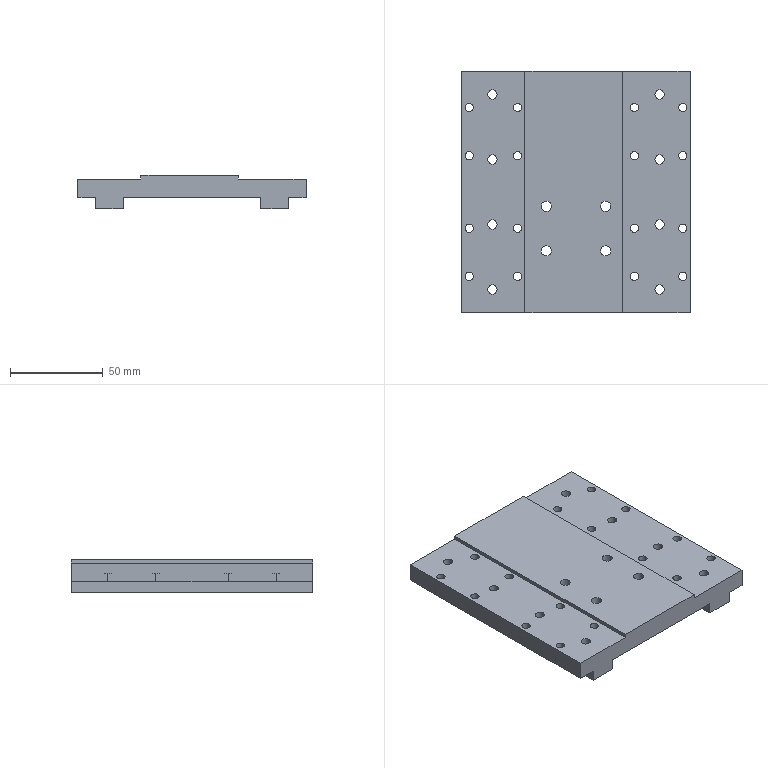NC program | NX | posted with a generic post | part box 123 x 130 x 18 mm
Lines 1 to 1849 of 2087, first 1534 of 1829 lines:
N10 G17 G21 G94 G90
(DRILLING , TOOL : D6A45)
N12 T01 M6
N14 G54
N16 G17 G0 G90 X-30.25 Y45.5 S5000 M3
N18 G43 Z30. H1
N20 G94 G81 G98 Z-1. F350. R3.
N22 X-43.75 Y52.5
N24 X-56.25 Y45.5
N26 Y19.5
N28 X-43.75 Y17.5
N30 X-30.25 Y19.5
N32 X-14.75 Y-7.7
N34 X-30.25 Y-19.5
N36 X-43.75 Y-17.5
N38 X-56.25 Y-19.5
N40 Y-45.5
N42 X-43.75 Y-52.5
N44 X-30.25 Y-45.5
N46 X-14.75 Y-31.7
N48 X17.25
N50 X32.75 Y-45.5
N52 X46.25 Y-52.5
N54 X58.75 Y-45.5
N56 Y-19.5
N58 X46.25 Y-17.5
N60 X32.75 Y-19.5
N62 X17.25 Y-7.7
N64 X32.75 Y19.5
N66 X46.25 Y17.5
N68 X58.75 Y19.5
N70 Y45.5
N72 X46.25 Y52.5
N74 X32.75 Y45.5
N76 G80
N78 G0 X32.75 Y45.5 Z30.
N80 M5
(DRILLING_COPY_COPY , TOOL : 5.5ZT)
N82 T09 M6
N84 G54
N86 G17 G0 G90 X-14.75 Y-7.7 S2000 M3
N88 G43 Z30. H9
N90 G94 G83 G98 Z-9.652 F300. Q2. R3.
N92 Y-31.7
N94 X17.25
N96 Y-7.7
N98 G80
N100 G0 X17.25 Y-7.7 Z30.
N102 M5
(DRILLING_COPY_COPY_COPY , TOOL : 5.0ZT)
N104 T16 M6
N106 G54
N108 G17 G0 G90 X46.25 Y-52.5 S2000 M3
N110 G43 Z30. H16
N112 G94 G83 G98 Z-21.002 F300. Q2. R3.
N114 Y-17.5
N116 Y17.5
N118 Y52.5
N120 X-43.75
N122 Y17.5
N124 Y-17.5
N126 Y-52.5
N128 G80
N130 G0 X-43.75 Y-52.5 Z30.
N132 M5
(DRILLING_COPY_COPY_COPY_COPY , TOOL : 4.5ZT)
N134 T08 M6
N136 G54
N138 G17 G0 G90 X32.75 Y-19.5 S2000 M3
N140 G43 Z30. H8
N142 G94 G83 G98 Z-10.352 F300. Q2. R3.
N144 Y-45.5
N146 X58.75
N148 Y-19.5
N150 Y19.5
N152 Y45.5
N154 X32.75
N156 Y19.5
N158 X-30.25
N160 Y45.5
N162 X-56.25
N164 Y19.5
N166 Y-19.5
N168 X-30.25
N170 Y-45.5
N172 X-56.25
N174 G80
N176 G0 X-56.25 Y-45.5 Z30.
N178 M5
(ZLEVEL_PROFILE , TOOL : D10)
N180 T15 M6
N182 G54
N184 G17 G0 G90 X-65.35 Y-47.067 S9500 M3
N186 G43 Z30. H15
N188 Z1.5
N190 G94 G1 Y0. Z-0.967 F1000.
N192 Y65. F3000.
N194 G2 X-60.25 Y70.1 R5.1
N196 G1 X62.75
N198 G2 X67.85 Y65. R5.1
N200 G1 Y-65.
N202 G2 X62.75 Y-70.1 R5.1
N204 G1 X-60.25
N206 G2 X-65.35 Y-65. R5.1
N208 G1 Y0.
N210 Y65. Z-1.083
N212 X-65.325 Y65.5 Z-1.084
N214 X-65.252 Y65.995 Z-1.085
N216 X-65.13 Y66.48 Z-1.086
N218 X-64.962 Y66.952 Z-1.087
N220 X-64.748 Y67.404 Z-1.088
N222 X-64.49 Y67.833 Z-1.089
N224 X-64.192 Y68.235 Z-1.09
N226 X-63.856 Y68.606 Z-1.091
N228 X-63.485 Y68.942 Z-1.092
N230 X-63.083 Y69.24
N232 X-62.654 Y69.498 Z-1.093
N234 X-62.202 Y69.712 Z-1.094
N236 X-61.73 Y69.88 Z-1.095
N238 X-61.245 Y70.002 Z-1.096
N240 X-60.75 Y70.075 Z-1.097
N242 X-60.25 Y70.1 Z-1.098
N244 X62.75 Z-1.319
N246 X63.25 Y70.075 Z-1.32
N248 X63.745 Y70.002 Z-1.321
N250 X64.23 Y69.88 Z-1.322
N252 X64.702 Y69.712
N254 X65.154 Y69.498 Z-1.323
N256 X65.583 Y69.24 Z-1.324
N258 X65.985 Y68.942 Z-1.325
N260 X66.356 Y68.606 Z-1.326
N262 X66.692 Y68.235 Z-1.327
N264 X66.99 Y67.833 Z-1.328
N266 X67.248 Y67.404 Z-1.329
N268 X67.462 Y66.952 Z-1.33
N270 X67.63 Y66.48 Z-1.331
N272 X67.752 Y65.995
N274 X67.825 Y65.5 Z-1.332
N276 X67.85 Y65. Z-1.333
N278 Y-65. Z-1.567
N280 X67.825 Y-65.5 Z-1.568
N282 X67.752 Y-65.995 Z-1.569
N284 X67.63 Y-66.48
N286 X67.462 Y-66.952 Z-1.57
N288 X67.248 Y-67.404 Z-1.571
N290 X66.99 Y-67.833 Z-1.572
N292 X66.692 Y-68.235 Z-1.573
N294 X66.356 Y-68.606 Z-1.574
N296 X65.985 Y-68.942 Z-1.575
N298 X65.583 Y-69.24 Z-1.576
N300 X65.154 Y-69.498 Z-1.577
N302 X64.702 Y-69.712 Z-1.578
N304 X64.23 Y-69.88
N306 X63.745 Y-70.002 Z-1.579
N308 X63.25 Y-70.075 Z-1.58
N310 X62.75 Y-70.1 Z-1.581
N312 X-60.25 Z-1.802
N314 X-60.75 Y-70.075 Z-1.803
N316 X-61.245 Y-70.002 Z-1.804
N318 X-61.73 Y-69.88 Z-1.805
N320 X-62.202 Y-69.712 Z-1.806
N322 X-62.654 Y-69.498 Z-1.807
N324 X-63.083 Y-69.24 Z-1.808
N326 X-63.485 Y-68.942
N328 X-63.856 Y-68.606 Z-1.809
N330 X-64.192 Y-68.235 Z-1.81
N332 X-64.49 Y-67.833 Z-1.811
N334 X-64.748 Y-67.404 Z-1.812
N336 X-64.962 Y-66.952 Z-1.813
N338 X-65.13 Y-66.48 Z-1.814
N340 X-65.252 Y-65.995 Z-1.815
N342 X-65.325 Y-65.5 Z-1.816
N344 X-65.35 Y-65. Z-1.817
N346 Y0. Z-1.933
N348 Y65. Z-2.05
N350 X-65.325 Y65.5 Z-2.051
N352 X-65.252 Y65.995 Z-2.052
N354 X-65.13 Y66.48 Z-2.053
N356 X-64.962 Y66.952 Z-2.054
N358 X-64.748 Y67.404 Z-2.055
N360 X-64.49 Y67.833 Z-2.056
N362 X-64.192 Y68.235
N364 X-63.856 Y68.606 Z-2.057
N366 X-63.485 Y68.942 Z-2.058
N368 X-63.083 Y69.24 Z-2.059
N370 X-62.654 Y69.498 Z-2.06
N372 X-62.202 Y69.712 Z-2.061
N374 X-61.73 Y69.88 Z-2.062
N376 X-61.245 Y70.002 Z-2.063
N378 X-60.75 Y70.075 Z-2.064
N380 X-60.25 Y70.1
N382 X62.75 Z-2.286
N384 X63.25 Y70.075
N386 X63.745 Y70.002 Z-2.287
N388 X64.23 Y69.88 Z-2.288
N390 X64.702 Y69.712 Z-2.289
N392 X65.154 Y69.498 Z-2.29
N394 X65.583 Y69.24 Z-2.291
N396 X65.985 Y68.942 Z-2.292
N398 X66.356 Y68.606 Z-2.293
N400 X66.692 Y68.235 Z-2.294
N402 X66.99 Y67.833
N404 X67.248 Y67.404 Z-2.295
N406 X67.462 Y66.952 Z-2.296
N408 X67.63 Y66.48 Z-2.297
N410 X67.752 Y65.995 Z-2.298
N412 X67.825 Y65.5 Z-2.299
N414 X67.85 Y65. Z-2.3
N416 Y-65. Z-2.533
N418 X67.825 Y-65.5 Z-2.534
N420 X67.752 Y-65.995 Z-2.535
N422 X67.63 Y-66.48 Z-2.536
N424 X67.462 Y-66.952 Z-2.537
N426 X67.248 Y-67.404 Z-2.538
N428 X66.99 Y-67.833 Z-2.539
N430 X66.692 Y-68.235 Z-2.54
N432 X66.356 Y-68.606 Z-2.541
N434 X65.985 Y-68.942 Z-2.542
N436 X65.583 Y-69.24
N438 X65.154 Y-69.498 Z-2.543
N440 X64.702 Y-69.712 Z-2.544
N442 X64.23 Y-69.88 Z-2.545
N444 X63.745 Y-70.002 Z-2.546
N446 X63.25 Y-70.075 Z-2.547
N448 X62.75 Y-70.1 Z-2.548
N450 X-60.25 Z-2.769
N452 X-60.75 Y-70.075 Z-2.77
N454 X-61.245 Y-70.002 Z-2.771
N456 X-61.73 Y-69.88 Z-2.772
N458 X-62.202 Y-69.712
N460 X-62.654 Y-69.498 Z-2.773
N462 X-63.083 Y-69.24 Z-2.774
N464 X-63.485 Y-68.942 Z-2.775
N466 X-63.856 Y-68.606 Z-2.776
N468 X-64.192 Y-68.235 Z-2.777
N470 X-64.49 Y-67.833 Z-2.778
N472 X-64.748 Y-67.404 Z-2.779
N474 X-64.962 Y-66.952 Z-2.78
N476 X-65.13 Y-66.48 Z-2.781
N478 X-65.252 Y-65.995
N480 X-65.325 Y-65.5 Z-2.782
N482 X-65.35 Y-65. Z-2.783
N484 Y0. Z-2.9
N486 Y65. Z-3.017
N488 X-65.325 Y65.5 Z-3.018
N490 X-65.252 Y65.995 Z-3.019
N492 X-65.13 Y66.48
N494 X-64.962 Y66.952 Z-3.02
N496 X-64.748 Y67.404 Z-3.021
N498 X-64.49 Y67.833 Z-3.022
N500 X-64.192 Y68.235 Z-3.023
N502 X-63.856 Y68.606 Z-3.024
N504 X-63.485 Y68.942 Z-3.025
N506 X-63.083 Y69.24 Z-3.026
N508 X-62.654 Y69.498 Z-3.027
N510 X-62.202 Y69.712 Z-3.028
N512 X-61.73 Y69.88
N514 X-61.245 Y70.002 Z-3.029
N516 X-60.75 Y70.075 Z-3.03
N518 X-60.25 Y70.1 Z-3.031
N520 X62.75 Z-3.252
N522 X63.25 Y70.075 Z-3.253
N524 X63.745 Y70.002 Z-3.254
N526 X64.23 Y69.88 Z-3.255
N528 X64.702 Y69.712 Z-3.256
N530 X65.154 Y69.498 Z-3.257
N532 X65.583 Y69.24 Z-3.258
N534 X65.985 Y68.942
N536 X66.356 Y68.606 Z-3.259
N538 X66.692 Y68.235 Z-3.26
N540 X66.99 Y67.833 Z-3.261
N542 X67.248 Y67.404 Z-3.262
N544 X67.462 Y66.952 Z-3.263
N546 X67.63 Y66.48 Z-3.264
N548 X67.752 Y65.995 Z-3.265
N550 X67.825 Y65.5 Z-3.266
N552 X67.85 Y65. Z-3.267
N554 Y-65. Z-3.5
N556 X67.825 Y-65.5 Z-3.501
N558 X67.752 Y-65.995 Z-3.502
N560 X67.63 Y-66.48 Z-3.503
N562 X67.462 Y-66.952 Z-3.504
N564 X67.248 Y-67.404 Z-3.505
N566 X66.99 Y-67.833 Z-3.506
N568 X66.692 Y-68.235
N570 X66.356 Y-68.606 Z-3.507
N572 X65.985 Y-68.942 Z-3.508
N574 X65.583 Y-69.24 Z-3.509
N576 X65.154 Y-69.498 Z-3.51
N578 X64.702 Y-69.712 Z-3.511
N580 X64.23 Y-69.88 Z-3.512
N582 X63.745 Y-70.002 Z-3.513
N584 X63.25 Y-70.075 Z-3.514
N586 X62.75 Y-70.1
N588 X-60.25 Z-3.736
N590 X-60.75 Y-70.075
N592 X-61.245 Y-70.002 Z-3.737
N594 X-61.73 Y-69.88 Z-3.738
N596 X-62.202 Y-69.712 Z-3.739
N598 X-62.654 Y-69.498 Z-3.74
N600 X-63.083 Y-69.24 Z-3.741
N602 X-63.485 Y-68.942 Z-3.742
N604 X-63.856 Y-68.606 Z-3.743
N606 X-64.192 Y-68.235 Z-3.744
N608 X-64.49 Y-67.833
N610 X-64.748 Y-67.404 Z-3.745
N612 X-64.962 Y-66.952 Z-3.746
N614 X-65.13 Y-66.48 Z-3.747
N616 X-65.252 Y-65.995 Z-3.748
N618 X-65.325 Y-65.5 Z-3.749
N620 X-65.35 Y-65. Z-3.75
N622 Y0. Z-3.867
N624 Y65. Z-3.983
N626 X-65.325 Y65.5 Z-3.984
N628 X-65.252 Y65.995 Z-3.985
N630 X-65.13 Y66.48 Z-3.986
N632 X-64.962 Y66.952 Z-3.987
N634 X-64.748 Y67.404 Z-3.988
N636 X-64.49 Y67.833 Z-3.989
N638 X-64.192 Y68.235 Z-3.99
N640 X-63.856 Y68.606 Z-3.991
N642 X-63.485 Y68.942 Z-3.992
N644 X-63.083 Y69.24
N646 X-62.654 Y69.498 Z-3.993
N648 X-62.202 Y69.712 Z-3.994
N650 X-61.73 Y69.88 Z-3.995
N652 X-61.245 Y70.002 Z-3.996
N654 X-60.75 Y70.075 Z-3.997
N656 X-60.25 Y70.1 Z-3.998
N658 X62.75 Z-4.219
N660 X63.25 Y70.075 Z-4.22
N662 X63.745 Y70.002 Z-4.221
N664 X64.23 Y69.88 Z-4.222
N666 X64.702 Y69.712
N668 X65.154 Y69.498 Z-4.223
N670 X65.583 Y69.24 Z-4.224
N672 X65.985 Y68.942 Z-4.225
N674 X66.356 Y68.606 Z-4.226
N676 X66.692 Y68.235 Z-4.227
N678 X66.99 Y67.833 Z-4.228
N680 X67.248 Y67.404 Z-4.229
N682 X67.462 Y66.952 Z-4.23
N684 X67.63 Y66.48 Z-4.231
N686 X67.752 Y65.995
N688 X67.825 Y65.5 Z-4.232
N690 X67.85 Y65. Z-4.233
N692 Y-65. Z-4.467
N694 X67.825 Y-65.5 Z-4.468
N696 X67.752 Y-65.995 Z-4.469
N698 X67.63 Y-66.48
N700 X67.462 Y-66.952 Z-4.47
N702 X67.248 Y-67.404 Z-4.471
N704 X66.99 Y-67.833 Z-4.472
N706 X66.692 Y-68.235 Z-4.473
N708 X66.356 Y-68.606 Z-4.474
N710 X65.985 Y-68.942 Z-4.475
N712 X65.583 Y-69.24 Z-4.476
N714 X65.154 Y-69.498 Z-4.477
N716 X64.702 Y-69.712 Z-4.478
N718 X64.23 Y-69.88
N720 X63.745 Y-70.002 Z-4.479
N722 X63.25 Y-70.075 Z-4.48
N724 X62.75 Y-70.1 Z-4.481
N726 X-60.25 Z-4.702
N728 X-60.75 Y-70.075 Z-4.703
N730 X-61.245 Y-70.002 Z-4.704
N732 X-61.73 Y-69.88 Z-4.705
N734 X-62.202 Y-69.712 Z-4.706
N736 X-62.654 Y-69.498 Z-4.707
N738 X-63.083 Y-69.24 Z-4.708
N740 X-63.485 Y-68.942
N742 X-63.856 Y-68.606 Z-4.709
N744 X-64.192 Y-68.235 Z-4.71
N746 X-64.49 Y-67.833 Z-4.711
N748 X-64.748 Y-67.404 Z-4.712
N750 X-64.962 Y-66.952 Z-4.713
N752 X-65.13 Y-66.48 Z-4.714
N754 X-65.252 Y-65.995 Z-4.715
N756 X-65.325 Y-65.5 Z-4.716
N758 X-65.35 Y-65. Z-4.717
N760 Y0. Z-4.833
N762 Y65. Z-4.95
N764 X-65.325 Y65.5 Z-4.951
N766 X-65.252 Y65.995 Z-4.952
N768 X-65.13 Y66.48 Z-4.953
N770 X-64.962 Y66.952 Z-4.954
N772 X-64.748 Y67.404 Z-4.955
N774 X-64.49 Y67.833 Z-4.956
N776 X-64.192 Y68.235
N778 X-63.856 Y68.606 Z-4.957
N780 X-63.485 Y68.942 Z-4.958
N782 X-63.083 Y69.24 Z-4.959
N784 X-62.654 Y69.498 Z-4.96
N786 X-62.202 Y69.712 Z-4.961
N788 X-61.73 Y69.88 Z-4.962
N790 X-61.245 Y70.002 Z-4.963
N792 X-60.75 Y70.075 Z-4.964
N794 X-60.25 Y70.1
N796 X62.75 Z-5.186
N798 X63.25 Y70.075
N800 X63.745 Y70.002 Z-5.187
N802 X64.23 Y69.88 Z-5.188
N804 X64.702 Y69.712 Z-5.189
N806 X65.154 Y69.498 Z-5.19
N808 X65.583 Y69.24 Z-5.191
N810 X65.985 Y68.942 Z-5.192
N812 X66.356 Y68.606 Z-5.193
N814 X66.692 Y68.235 Z-5.194
N816 X66.99 Y67.833
N818 X67.248 Y67.404 Z-5.195
N820 X67.462 Y66.952 Z-5.196
N822 X67.63 Y66.48 Z-5.197
N824 X67.752 Y65.995 Z-5.198
N826 X67.825 Y65.5 Z-5.199
N828 X67.85 Y65. Z-5.2
N830 Y-65. Z-5.433
N832 X67.825 Y-65.5 Z-5.434
N834 X67.752 Y-65.995 Z-5.435
N836 X67.63 Y-66.48 Z-5.436
N838 X67.462 Y-66.952 Z-5.437
N840 X67.248 Y-67.404 Z-5.438
N842 X66.99 Y-67.833 Z-5.439
N844 X66.692 Y-68.235 Z-5.44
N846 X66.356 Y-68.606 Z-5.441
N848 X65.985 Y-68.942 Z-5.442
N850 X65.583 Y-69.24
N852 X65.154 Y-69.498 Z-5.443
N854 X64.702 Y-69.712 Z-5.444
N856 X64.23 Y-69.88 Z-5.445
N858 X63.745 Y-70.002 Z-5.446
N860 X63.25 Y-70.075 Z-5.447
N862 X62.75 Y-70.1 Z-5.448
N864 X-60.25 Z-5.669
N866 X-60.75 Y-70.075 Z-5.67
N868 X-61.245 Y-70.002 Z-5.671
N870 X-61.73 Y-69.88 Z-5.672
N872 X-62.202 Y-69.712
N874 X-62.654 Y-69.498 Z-5.673
N876 X-63.083 Y-69.24 Z-5.674
N878 X-63.485 Y-68.942 Z-5.675
N880 X-63.856 Y-68.606 Z-5.676
N882 X-64.192 Y-68.235 Z-5.677
N884 X-64.49 Y-67.833 Z-5.678
N886 X-64.748 Y-67.404 Z-5.679
N888 X-64.962 Y-66.952 Z-5.68
N890 X-65.13 Y-66.48 Z-5.681
N892 X-65.252 Y-65.995
N894 X-65.325 Y-65.5 Z-5.682
N896 X-65.35 Y-65. Z-5.683
N898 Y0. Z-5.8
N900 Y65. Z-5.917
N902 X-65.325 Y65.5 Z-5.918
N904 X-65.252 Y65.995 Z-5.919
N906 X-65.13 Y66.48
N908 X-64.962 Y66.952 Z-5.92
N910 X-64.748 Y67.404 Z-5.921
N912 X-64.49 Y67.833 Z-5.922
N914 X-64.192 Y68.235 Z-5.923
N916 X-63.856 Y68.606 Z-5.924
N918 X-63.485 Y68.942 Z-5.925
N920 X-63.083 Y69.24 Z-5.926
N922 X-62.654 Y69.498 Z-5.927
N924 X-62.202 Y69.712 Z-5.928
N926 X-61.73 Y69.88
N928 X-61.245 Y70.002 Z-5.929
N930 X-60.75 Y70.075 Z-5.93
N932 X-60.25 Y70.1 Z-5.931
N934 X62.75 Z-6.152
N936 X63.25 Y70.075 Z-6.153
N938 X63.745 Y70.002 Z-6.154
N940 X64.23 Y69.88 Z-6.155
N942 X64.702 Y69.712 Z-6.156
N944 X65.154 Y69.498 Z-6.157
N946 X65.583 Y69.24 Z-6.158
N948 X65.985 Y68.942
N950 X66.356 Y68.606 Z-6.159
N952 X66.692 Y68.235 Z-6.16
N954 X66.99 Y67.833 Z-6.161
N956 X67.248 Y67.404 Z-6.162
N958 X67.462 Y66.952 Z-6.163
N960 X67.63 Y66.48 Z-6.164
N962 X67.752 Y65.995 Z-6.165
N964 X67.825 Y65.5 Z-6.166
N966 X67.85 Y65. Z-6.167
N968 Y-65. Z-6.4
N970 X67.825 Y-65.5 Z-6.401
N972 X67.752 Y-65.995 Z-6.402
N974 X67.63 Y-66.48 Z-6.403
N976 X67.462 Y-66.952 Z-6.404
N978 X67.248 Y-67.404 Z-6.405
N980 X66.99 Y-67.833 Z-6.406
N982 X66.692 Y-68.235
N984 X66.356 Y-68.606 Z-6.407
N986 X65.985 Y-68.942 Z-6.408
N988 X65.583 Y-69.24 Z-6.409
N990 X65.154 Y-69.498 Z-6.41
N992 X64.702 Y-69.712 Z-6.411
N994 X64.23 Y-69.88 Z-6.412
N996 X63.745 Y-70.002 Z-6.413
N998 X63.25 Y-70.075 Z-6.414
N1000 X62.75 Y-70.1
N1002 X-60.25 Z-6.636
N1004 X-60.75 Y-70.075
N1006 X-61.245 Y-70.002 Z-6.637
N1008 X-61.73 Y-69.88 Z-6.638
N1010 X-62.202 Y-69.712 Z-6.639
N1012 X-62.654 Y-69.498 Z-6.64
N1014 X-63.083 Y-69.24 Z-6.641
N1016 X-63.485 Y-68.942 Z-6.642
N1018 X-63.856 Y-68.606 Z-6.643
N1020 X-64.192 Y-68.235 Z-6.644
N1022 X-64.49 Y-67.833
N1024 X-64.748 Y-67.404 Z-6.645
N1026 X-64.962 Y-66.952 Z-6.646
N1028 X-65.13 Y-66.48 Z-6.647
N1030 X-65.252 Y-65.995 Z-6.648
N1032 X-65.325 Y-65.5 Z-6.649
N1034 X-65.35 Y-65. Z-6.65
N1036 Y0. Z-6.767
N1038 Y65. Z-6.883
N1040 X-65.325 Y65.5 Z-6.884
N1042 X-65.252 Y65.995 Z-6.885
N1044 X-65.13 Y66.48 Z-6.886
N1046 X-64.962 Y66.952 Z-6.887
N1048 X-64.748 Y67.404 Z-6.888
N1050 X-64.49 Y67.833 Z-6.889
N1052 X-64.192 Y68.235 Z-6.89
N1054 X-63.856 Y68.606 Z-6.891
N1056 X-63.485 Y68.942 Z-6.892
N1058 X-63.083 Y69.24
N1060 X-62.654 Y69.498 Z-6.893
N1062 X-62.202 Y69.712 Z-6.894
N1064 X-61.73 Y69.88 Z-6.895
N1066 X-61.245 Y70.002 Z-6.896
N1068 X-60.75 Y70.075 Z-6.897
N1070 X-60.25 Y70.1 Z-6.898
N1072 X62.75 Z-7.119
N1074 X63.25 Y70.075 Z-7.12
N1076 X63.745 Y70.002 Z-7.121
N1078 X64.23 Y69.88 Z-7.122
N1080 X64.702 Y69.712
N1082 X65.154 Y69.498 Z-7.123
N1084 X65.583 Y69.24 Z-7.124
N1086 X65.985 Y68.942 Z-7.125
N1088 X66.356 Y68.606 Z-7.126
N1090 X66.692 Y68.235 Z-7.127
N1092 X66.99 Y67.833 Z-7.128
N1094 X67.248 Y67.404 Z-7.129
N1096 X67.462 Y66.952 Z-7.13
N1098 X67.63 Y66.48 Z-7.131
N1100 X67.752 Y65.995
N1102 X67.825 Y65.5 Z-7.132
N1104 X67.85 Y65. Z-7.133
N1106 Y-65. Z-7.367
N1108 X67.825 Y-65.5 Z-7.368
N1110 X67.752 Y-65.995 Z-7.369
N1112 X67.63 Y-66.48
N1114 X67.462 Y-66.952 Z-7.37
N1116 X67.248 Y-67.404 Z-7.371
N1118 X66.99 Y-67.833 Z-7.372
N1120 X66.692 Y-68.235 Z-7.373
N1122 X66.356 Y-68.606 Z-7.374
N1124 X65.985 Y-68.942 Z-7.375
N1126 X65.583 Y-69.24 Z-7.376
N1128 X65.154 Y-69.498 Z-7.377
N1130 X64.702 Y-69.712 Z-7.378
N1132 X64.23 Y-69.88
N1134 X63.745 Y-70.002 Z-7.379
N1136 X63.25 Y-70.075 Z-7.38
N1138 X62.75 Y-70.1 Z-7.381
N1140 X-60.25 Z-7.602
N1142 X-60.75 Y-70.075 Z-7.603
N1144 X-61.245 Y-70.002 Z-7.604
N1146 X-61.73 Y-69.88 Z-7.605
N1148 X-62.202 Y-69.712 Z-7.606
N1150 X-62.654 Y-69.498 Z-7.607
N1152 X-63.083 Y-69.24 Z-7.608
N1154 X-63.485 Y-68.942
N1156 X-63.856 Y-68.606 Z-7.609
N1158 X-64.192 Y-68.235 Z-7.61
N1160 X-64.49 Y-67.833 Z-7.611
N1162 X-64.748 Y-67.404 Z-7.612
N1164 X-64.962 Y-66.952 Z-7.613
N1166 X-65.13 Y-66.48 Z-7.614
N1168 X-65.252 Y-65.995 Z-7.615
N1170 X-65.325 Y-65.5 Z-7.616
N1172 X-65.35 Y-65. Z-7.617
N1174 Y0. Z-7.733
N1176 Y65. Z-7.85
N1178 X-65.325 Y65.5 Z-7.851
N1180 X-65.252 Y65.995 Z-7.852
N1182 X-65.13 Y66.48 Z-7.853
N1184 X-64.962 Y66.952 Z-7.854
N1186 X-64.748 Y67.404 Z-7.855
N1188 X-64.49 Y67.833 Z-7.856
N1190 X-64.192 Y68.235
N1192 X-63.856 Y68.606 Z-7.857
N1194 X-63.485 Y68.942 Z-7.858
N1196 X-63.083 Y69.24 Z-7.859
N1198 X-62.654 Y69.498 Z-7.86
N1200 X-62.202 Y69.712 Z-7.861
N1202 X-61.73 Y69.88 Z-7.862
N1204 X-61.245 Y70.002 Z-7.863
N1206 X-60.75 Y70.075 Z-7.864
N1208 X-60.25 Y70.1
N1210 X62.75 Z-8.086
N1212 X63.25 Y70.075
N1214 X63.745 Y70.002 Z-8.087
N1216 X64.23 Y69.88 Z-8.088
N1218 X64.702 Y69.712 Z-8.089
N1220 X65.154 Y69.498 Z-8.09
N1222 X65.583 Y69.24 Z-8.091
N1224 X65.985 Y68.942 Z-8.092
N1226 X66.356 Y68.606 Z-8.093
N1228 X66.692 Y68.235 Z-8.094
N1230 X66.99 Y67.833
N1232 X67.248 Y67.404 Z-8.095
N1234 X67.462 Y66.952 Z-8.096
N1236 X67.63 Y66.48 Z-8.097
N1238 X67.752 Y65.995 Z-8.098
N1240 X67.825 Y65.5 Z-8.099
N1242 X67.85 Y65. Z-8.1
N1244 Y-65. Z-8.333
N1246 X67.825 Y-65.5 Z-8.334
N1248 X67.752 Y-65.995 Z-8.335
N1250 X67.63 Y-66.48 Z-8.336
N1252 X67.462 Y-66.952 Z-8.337
N1254 X67.248 Y-67.404 Z-8.338
N1256 X66.99 Y-67.833 Z-8.339
N1258 X66.692 Y-68.235 Z-8.34
N1260 X66.356 Y-68.606 Z-8.341
N1262 X65.985 Y-68.942 Z-8.342
N1264 X65.583 Y-69.24
N1266 X65.154 Y-69.498 Z-8.343
N1268 X64.702 Y-69.712 Z-8.344
N1270 X64.23 Y-69.88 Z-8.345
N1272 X63.745 Y-70.002 Z-8.346
N1274 X63.25 Y-70.075 Z-8.347
N1276 X62.75 Y-70.1 Z-8.348
N1278 X-60.25 Z-8.569
N1280 X-60.75 Y-70.075 Z-8.57
N1282 X-61.245 Y-70.002 Z-8.571
N1284 X-61.73 Y-69.88 Z-8.572
N1286 X-62.202 Y-69.712
N1288 X-62.654 Y-69.498 Z-8.573
N1290 X-63.083 Y-69.24 Z-8.574
N1292 X-63.485 Y-68.942 Z-8.575
N1294 X-63.856 Y-68.606 Z-8.576
N1296 X-64.192 Y-68.235 Z-8.577
N1298 X-64.49 Y-67.833 Z-8.578
N1300 X-64.748 Y-67.404 Z-8.579
N1302 X-64.962 Y-66.952 Z-8.58
N1304 X-65.13 Y-66.48 Z-8.581
N1306 X-65.252 Y-65.995
N1308 X-65.325 Y-65.5 Z-8.582
N1310 X-65.35 Y-65. Z-8.583
N1312 Y0. Z-8.7
N1314 Y65. Z-8.817
N1316 X-65.325 Y65.5 Z-8.818
N1318 X-65.252 Y65.995 Z-8.819
N1320 X-65.13 Y66.48
N1322 X-64.962 Y66.952 Z-8.82
N1324 X-64.748 Y67.404 Z-8.821
N1326 X-64.49 Y67.833 Z-8.822
N1328 X-64.192 Y68.235 Z-8.823
N1330 X-63.856 Y68.606 Z-8.824
N1332 X-63.485 Y68.942 Z-8.825
N1334 X-63.083 Y69.24 Z-8.826
N1336 X-62.654 Y69.498 Z-8.827
N1338 X-62.202 Y69.712 Z-8.828
N1340 X-61.73 Y69.88
N1342 X-61.245 Y70.002 Z-8.829
N1344 X-60.75 Y70.075 Z-8.83
N1346 X-60.25 Y70.1 Z-8.831
N1348 X62.75 Z-9.052
N1350 X63.25 Y70.075 Z-9.053
N1352 X63.745 Y70.002 Z-9.054
N1354 X64.23 Y69.88 Z-9.055
N1356 X64.702 Y69.712 Z-9.056
N1358 X65.154 Y69.498 Z-9.057
N1360 X65.583 Y69.24 Z-9.058
N1362 X65.985 Y68.942
N1364 X66.356 Y68.606 Z-9.059
N1366 X66.692 Y68.235 Z-9.06
N1368 X66.99 Y67.833 Z-9.061
N1370 X67.248 Y67.404 Z-9.062
N1372 X67.462 Y66.952 Z-9.063
N1374 X67.63 Y66.48 Z-9.064
N1376 X67.752 Y65.995 Z-9.065
N1378 X67.825 Y65.5 Z-9.066
N1380 X67.85 Y65. Z-9.067
N1382 Y-65. Z-9.3
N1384 X67.825 Y-65.5 Z-9.301
N1386 X67.752 Y-65.995 Z-9.302
N1388 X67.63 Y-66.48 Z-9.303
N1390 X67.462 Y-66.952 Z-9.304
N1392 X67.248 Y-67.404 Z-9.305
N1394 X66.99 Y-67.833 Z-9.306
N1396 X66.692 Y-68.235
N1398 X66.356 Y-68.606 Z-9.307
N1400 X65.985 Y-68.942 Z-9.308
N1402 X65.583 Y-69.24 Z-9.309
N1404 X65.154 Y-69.498 Z-9.31
N1406 X64.702 Y-69.712 Z-9.311
N1408 X64.23 Y-69.88 Z-9.312
N1410 X63.745 Y-70.002 Z-9.313
N1412 X63.25 Y-70.075 Z-9.314
N1414 X62.75 Y-70.1
N1416 X-60.25 Z-9.536
N1418 X-60.75 Y-70.075
N1420 X-61.245 Y-70.002 Z-9.537
N1422 X-61.73 Y-69.88 Z-9.538
N1424 X-62.202 Y-69.712 Z-9.539
N1426 X-62.654 Y-69.498 Z-9.54
N1428 X-63.083 Y-69.24 Z-9.541
N1430 X-63.485 Y-68.942 Z-9.542
N1432 X-63.856 Y-68.606 Z-9.543
N1434 X-64.192 Y-68.235 Z-9.544
N1436 X-64.49 Y-67.833
N1438 X-64.748 Y-67.404 Z-9.545
N1440 X-64.962 Y-66.952 Z-9.546
N1442 X-65.13 Y-66.48 Z-9.547
N1444 X-65.252 Y-65.995 Z-9.548
N1446 X-65.325 Y-65.5 Z-9.549
N1448 X-65.35 Y-65. Z-9.55
N1450 Y0. Z-9.667
N1452 Y65. Z-9.783
N1454 X-65.325 Y65.5 Z-9.784
N1456 X-65.252 Y65.995 Z-9.785
N1458 X-65.13 Y66.48 Z-9.786
N1460 X-64.962 Y66.952 Z-9.787
N1462 X-64.748 Y67.404 Z-9.788
N1464 X-64.49 Y67.833 Z-9.789
N1466 X-64.192 Y68.235 Z-9.79
N1468 X-63.856 Y68.606 Z-9.791
N1470 X-63.485 Y68.942 Z-9.792
N1472 X-63.083 Y69.24
N1474 X-62.654 Y69.498 Z-9.793
N1476 X-62.202 Y69.712 Z-9.794
N1478 X-61.73 Y69.88 Z-9.795
N1480 X-61.245 Y70.002 Z-9.796
N1482 X-60.75 Y70.075 Z-9.797
N1484 X-60.25 Y70.1 Z-9.798
N1486 X62.75 Z-10.019
N1488 X63.25 Y70.075 Z-10.02
N1490 X63.745 Y70.002 Z-10.021
N1492 X64.23 Y69.88 Z-10.022
N1494 X64.702 Y69.712
N1496 X65.154 Y69.498 Z-10.023
N1498 X65.583 Y69.24 Z-10.024
N1500 X65.985 Y68.942 Z-10.025
N1502 X66.356 Y68.606 Z-10.026
N1504 X66.692 Y68.235 Z-10.027
N1506 X66.99 Y67.833 Z-10.028
N1508 X67.248 Y67.404 Z-10.029
N1510 X67.462 Y66.952 Z-10.03
N1512 X67.63 Y66.48 Z-10.031
N1514 X67.752 Y65.995
N1516 X67.825 Y65.5 Z-10.032
N1518 X67.85 Y65. Z-10.033
N1520 Y-65. Z-10.267
N1522 X67.825 Y-65.5 Z-10.268
N1524 X67.752 Y-65.995 Z-10.269
N1526 X67.63 Y-66.48
N1528 X67.462 Y-66.952 Z-10.27
N1530 X67.248 Y-67.404 Z-10.271
N1532 X66.99 Y-67.833 Z-10.272
N1534 X66.692 Y-68.235 Z-10.273
N1536 X66.356 Y-68.606 Z-10.274
N1538 X65.985 Y-68.942 Z-10.275
N1540 X65.583 Y-69.24 Z-10.276
N1542 X65.154 Y-69.498 Z-10.277
N1544 X64.702 Y-69.712 Z-10.278
N1546 X64.23 Y-69.88
N1548 X63.745 Y-70.002 Z-10.279
N1550 X63.25 Y-70.075 Z-10.28
N1552 X62.75 Y-70.1 Z-10.281
N1554 X-60.25 Z-10.502
N1556 X-60.75 Y-70.075 Z-10.503
N1558 X-61.245 Y-70.002 Z-10.504
N1560 X-61.73 Y-69.88 Z-10.505
N1562 X-62.202 Y-69.712 Z-10.506
N1564 X-62.654 Y-69.498 Z-10.507
N1566 X-63.083 Y-69.24 Z-10.508
N1568 X-63.485 Y-68.942
N1570 X-63.856 Y-68.606 Z-10.509
N1572 X-64.192 Y-68.235 Z-10.51
N1574 X-64.49 Y-67.833 Z-10.511
N1576 X-64.748 Y-67.404 Z-10.512
N1578 X-64.962 Y-66.952 Z-10.513
N1580 X-65.13 Y-66.48 Z-10.514
N1582 X-65.252 Y-65.995 Z-10.515
N1584 X-65.325 Y-65.5 Z-10.516
N1586 X-65.35 Y-65. Z-10.517
N1588 Y0. Z-10.633
N1590 Y65. Z-10.75
N1592 X-65.325 Y65.5 Z-10.751
N1594 X-65.252 Y65.995 Z-10.752
N1596 X-65.13 Y66.48 Z-10.753
N1598 X-64.962 Y66.952 Z-10.754
N1600 X-64.748 Y67.404 Z-10.755
N1602 X-64.49 Y67.833 Z-10.756
N1604 X-64.192 Y68.235
N1606 X-63.856 Y68.606 Z-10.757
N1608 X-63.485 Y68.942 Z-10.758
N1610 X-63.083 Y69.24 Z-10.759
N1612 X-62.654 Y69.498 Z-10.76
N1614 X-62.202 Y69.712 Z-10.761
N1616 X-61.73 Y69.88 Z-10.762
N1618 X-61.245 Y70.002 Z-10.763
N1620 X-60.75 Y70.075 Z-10.764
N1622 X-60.25 Y70.1
N1624 X62.75 Z-10.986
N1626 X63.25 Y70.075
N1628 X63.745 Y70.002 Z-10.987
N1630 X64.23 Y69.88 Z-10.988
N1632 X64.702 Y69.712 Z-10.989
N1634 X65.154 Y69.498 Z-10.99
N1636 X65.583 Y69.24 Z-10.991
N1638 X65.985 Y68.942 Z-10.992
N1640 X66.356 Y68.606 Z-10.993
N1642 X66.692 Y68.235 Z-10.994
N1644 X66.99 Y67.833
N1646 X67.248 Y67.404 Z-10.995
N1648 X67.462 Y66.952 Z-10.996
N1650 X67.63 Y66.48 Z-10.997
N1652 X67.752 Y65.995 Z-10.998
N1654 X67.825 Y65.5 Z-10.999
N1656 X67.85 Y65. Z-11.
N1658 Y-65. Z-11.233
N1660 X67.825 Y-65.5 Z-11.234
N1662 X67.752 Y-65.995 Z-11.235
N1664 X67.63 Y-66.48 Z-11.236
N1666 X67.462 Y-66.952 Z-11.237
N1668 X67.248 Y-67.404 Z-11.238
N1670 X66.99 Y-67.833 Z-11.239
N1672 X66.692 Y-68.235 Z-11.24
N1674 X66.356 Y-68.606 Z-11.241
N1676 X65.985 Y-68.942 Z-11.242
N1678 X65.583 Y-69.24
N1680 X65.154 Y-69.498 Z-11.243
N1682 X64.702 Y-69.712 Z-11.244
N1684 X64.23 Y-69.88 Z-11.245
N1686 X63.745 Y-70.002 Z-11.246
N1688 X63.25 Y-70.075 Z-11.247
N1690 X62.75 Y-70.1 Z-11.248
N1692 X-60.25 Z-11.469
N1694 X-60.75 Y-70.075 Z-11.47
N1696 X-61.245 Y-70.002 Z-11.471
N1698 X-61.73 Y-69.88 Z-11.472
N1700 X-62.202 Y-69.712
N1702 X-62.654 Y-69.498 Z-11.473
N1704 X-63.083 Y-69.24 Z-11.474
N1706 X-63.485 Y-68.942 Z-11.475
N1708 X-63.856 Y-68.606 Z-11.476
N1710 X-64.192 Y-68.235 Z-11.477
N1712 X-64.49 Y-67.833 Z-11.478
N1714 X-64.748 Y-67.404 Z-11.479
N1716 X-64.962 Y-66.952 Z-11.48
N1718 X-65.13 Y-66.48 Z-11.481
N1720 X-65.252 Y-65.995
N1722 X-65.325 Y-65.5 Z-11.482
N1724 X-65.35 Y-65. Z-11.483
N1726 Y0. Z-11.6
N1728 Y65. Z-11.717
N1730 X-65.325 Y65.5 Z-11.718
N1732 X-65.252 Y65.995 Z-11.719
N1734 X-65.13 Y66.48
N1736 X-64.962 Y66.952 Z-11.72
N1738 X-64.748 Y67.404 Z-11.721
N1740 X-64.49 Y67.833 Z-11.722
N1742 X-64.192 Y68.235 Z-11.723
N1744 X-63.856 Y68.606 Z-11.724
N1746 X-63.485 Y68.942 Z-11.725
N1748 X-63.083 Y69.24 Z-11.726
N1750 X-62.654 Y69.498 Z-11.727
N1752 X-62.202 Y69.712 Z-11.728
N1754 X-61.73 Y69.88
N1756 X-61.245 Y70.002 Z-11.729
N1758 X-60.75 Y70.075 Z-11.73
N1760 X-60.25 Y70.1 Z-11.731
N1762 X62.75 Z-11.952
N1764 X63.25 Y70.075 Z-11.953
N1766 X63.745 Y70.002 Z-11.954
N1768 X64.23 Y69.88 Z-11.955
N1770 X64.702 Y69.712 Z-11.956
N1772 X65.154 Y69.498 Z-11.957
N1774 X65.583 Y69.24 Z-11.958
N1776 X65.985 Y68.942
N1778 X66.356 Y68.606 Z-11.959
N1780 X66.692 Y68.235 Z-11.96
N1782 X66.99 Y67.833 Z-11.961
N1784 X67.248 Y67.404 Z-11.962
N1786 X67.462 Y66.952 Z-11.963
N1788 X67.63 Y66.48 Z-11.964
N1790 X67.752 Y65.995 Z-11.965
N1792 X67.825 Y65.5 Z-11.966
N1794 X67.85 Y65. Z-11.967
N1796 Y-65. Z-12.2
N1798 X67.825 Y-65.5 Z-12.201
N1800 X67.752 Y-65.995 Z-12.202
N1802 X67.63 Y-66.48 Z-12.203
N1804 X67.462 Y-66.952 Z-12.204
N1806 X67.248 Y-67.404 Z-12.205
N1808 X66.99 Y-67.833 Z-12.206
N1810 X66.692 Y-68.235
N1812 X66.356 Y-68.606 Z-12.207
N1814 X65.985 Y-68.942 Z-12.208
N1816 X65.583 Y-69.24 Z-12.209
N1818 X65.154 Y-69.498 Z-12.21
N1820 X64.702 Y-69.712 Z-12.211
N1822 X64.23 Y-69.88 Z-12.212
N1824 X63.745 Y-70.002 Z-12.213
N1826 X63.25 Y-70.075 Z-12.214
N1828 X62.75 Y-70.1
N1830 X-60.25 Z-12.436
N1832 X-60.75 Y-70.075
N1834 X-61.245 Y-70.002 Z-12.437
N1836 X-61.73 Y-69.88 Z-12.438
N1838 X-62.202 Y-69.712 Z-12.439
N1840 X-62.654 Y-69.498 Z-12.44
N1842 X-63.083 Y-69.24 Z-12.441
N1844 X-63.485 Y-68.942 Z-12.442
N1846 X-63.856 Y-68.606 Z-12.443
N1848 X-64.192 Y-68.235 Z-12.444
N1850 X-64.49 Y-67.833
N1852 X-64.748 Y-67.404 Z-12.445
N1854 X-64.962 Y-66.952 Z-12.446
N1856 X-65.13 Y-66.48 Z-12.447
N1858 X-65.252 Y-65.995 Z-12.448
N1860 X-65.325 Y-65.5 Z-12.449
N1862 X-65.35 Y-65. Z-12.45
N1864 Y0. Z-12.567
N1866 Y65. Z-12.683
N1868 X-65.325 Y65.5 Z-12.684
N1870 X-65.252 Y65.995 Z-12.685
N1872 X-65.13 Y66.48 Z-12.686
N1874 X-64.962 Y66.952 Z-12.687
N1876 X-64.748 Y67.404 Z-12.688
N1878 X-64.49 Y67.833 Z-12.689
N1880 X-64.192 Y68.235 Z-12.69
N1882 X-63.856 Y68.606 Z-12.691
N1884 X-63.485 Y68.942 Z-12.692
N1886 X-63.083 Y69.24
N1888 X-62.654 Y69.498 Z-12.693
N1890 X-62.202 Y69.712 Z-12.694
N1892 X-61.73 Y69.88 Z-12.695
N1894 X-61.245 Y70.002 Z-12.696
N1896 X-60.75 Y70.075 Z-12.697
N1898 X-60.25 Y70.1 Z-12.698
N1900 X62.75 Z-12.919
N1902 X63.25 Y70.075 Z-12.92
N1904 X63.745 Y70.002 Z-12.921
N1906 X64.23 Y69.88 Z-12.922
N1908 X64.702 Y69.712
N1910 X65.154 Y69.498 Z-12.923
N1912 X65.583 Y69.24 Z-12.924
N1914 X65.985 Y68.942 Z-12.925
N1916 X66.356 Y68.606 Z-12.926
N1918 X66.692 Y68.235 Z-12.927
N1920 X66.99 Y67.833 Z-12.928
N1922 X67.248 Y67.404 Z-12.929
N1924 X67.462 Y66.952 Z-12.93
N1926 X67.63 Y66.48 Z-12.931
N1928 X67.752 Y65.995
N1930 X67.825 Y65.5 Z-12.932
N1932 X67.85 Y65. Z-12.933
N1934 Y-65. Z-13.167
N1936 X67.825 Y-65.5 Z-13.168
N1938 X67.752 Y-65.995 Z-13.169
N1940 X67.63 Y-66.48
N1942 X67.462 Y-66.952 Z-13.17
N1944 X67.248 Y-67.404 Z-13.171
N1946 X66.99 Y-67.833 Z-13.172
N1948 X66.692 Y-68.235 Z-13.173
N1950 X66.356 Y-68.606 Z-13.174
N1952 X65.985 Y-68.942 Z-13.175
N1954 X65.583 Y-69.24 Z-13.176
N1956 X65.154 Y-69.498 Z-13.177
N1958 X64.702 Y-69.712 Z-13.178
N1960 X64.23 Y-69.88
N1962 X63.745 Y-70.002 Z-13.179
N1964 X63.25 Y-70.075 Z-13.18
N1966 X62.75 Y-70.1 Z-13.181
N1968 X-60.25 Z-13.402
N1970 X-60.75 Y-70.075 Z-13.403
N1972 X-61.245 Y-70.002 Z-13.404
N1974 X-61.73 Y-69.88 Z-13.405
N1976 X-62.202 Y-69.712 Z-13.406
N1978 X-62.654 Y-69.498 Z-13.407
N1980 X-63.083 Y-69.24 Z-13.408
N1982 X-63.485 Y-68.942
N1984 X-63.856 Y-68.606 Z-13.409
N1986 X-64.192 Y-68.235 Z-13.41
N1988 X-64.49 Y-67.833 Z-13.411
N1990 X-64.748 Y-67.404 Z-13.412
N1992 X-64.962 Y-66.952 Z-13.413
N1994 X-65.13 Y-66.48 Z-13.414
N1996 X-65.252 Y-65.995 Z-13.415
N1998 X-65.325 Y-65.5 Z-13.416
N2000 X-65.35 Y-65. Z-13.417
N2002 Y0. Z-13.533
N2004 Y65. Z-13.65
N2006 X-65.325 Y65.5 Z-13.651
N2008 X-65.252 Y65.995 Z-13.652
N2010 X-65.13 Y66.48 Z-13.653
N2012 X-64.962 Y66.952 Z-13.654
N2014 X-64.748 Y67.404 Z-13.655
N2016 X-64.49 Y67.833 Z-13.656
N2018 X-64.192 Y68.235
N2020 X-63.856 Y68.606 Z-13.657
N2022 X-63.485 Y68.942 Z-13.658
N2024 X-63.083 Y69.24 Z-13.659
N2026 X-62.654 Y69.498 Z-13.66
N2028 X-62.202 Y69.712 Z-13.661
N2030 X-61.73 Y69.88 Z-13.662
N2032 X-61.245 Y70.002 Z-13.663
N2034 X-60.75 Y70.075 Z-13.664
N2036 X-60.25 Y70.1
N2038 X62.75 Z-13.886
N2040 X63.25 Y70.075
N2042 X63.745 Y70.002 Z-13.887
N2044 X64.23 Y69.88 Z-13.888
N2046 X64.702 Y69.712 Z-13.889
N2048 X65.154 Y69.498 Z-13.89
N2050 X65.583 Y69.24 Z-13.891
N2052 X65.985 Y68.942 Z-13.892
N2054 X66.356 Y68.606 Z-13.893
N2056 X66.692 Y68.235 Z-13.894
N2058 X66.99 Y67.833
N2060 X67.248 Y67.404 Z-13.895
N2062 X67.462 Y66.952 Z-13.896
N2064 X67.63 Y66.48 Z-13.897
N2066 X67.752 Y65.995 Z-13.898
N2068 X67.825 Y65.5 Z-13.899
N2070 X67.85 Y65. Z-13.9
N2072 Y-65. Z-14.133
N2074 X67.825 Y-65.5 Z-14.134
N2076 X67.752 Y-65.995 Z-14.135
N2078 X67.63 Y-66.48 Z-14.136
N2080 X67.462 Y-66.952 Z-14.137
N2082 X67.248 Y-67.404 Z-14.138
N2084 X66.99 Y-67.833 Z-14.139
N2086 X66.692 Y-68.235 Z-14.14
N2088 X66.356 Y-68.606 Z-14.141
N2090 X65.985 Y-68.942 Z-14.142
N2092 X65.583 Y-69.24
N2094 X65.154 Y-69.498 Z-14.143
N2096 X64.702 Y-69.712 Z-14.144
N2098 X64.23 Y-69.88 Z-14.145
N2100 X63.745 Y-70.002 Z-14.146
N2102 X63.25 Y-70.075 Z-14.147
N2104 X62.75 Y-70.1 Z-14.148
N2106 X-60.25 Z-14.369
N2108 X-60.75 Y-70.075 Z-14.37
N2110 X-61.245 Y-70.002 Z-14.371
N2112 X-61.73 Y-69.88 Z-14.372
N2114 X-62.202 Y-69.712
N2116 X-62.654 Y-69.498 Z-14.373
N2118 X-63.083 Y-69.24 Z-14.374
N2120 X-63.485 Y-68.942 Z-14.375
N2122 X-63.856 Y-68.606 Z-14.376
N2124 X-64.192 Y-68.235 Z-14.377
N2126 X-64.49 Y-67.833 Z-14.378
N2128 X-64.748 Y-67.404 Z-14.379
N2130 X-64.962 Y-66.952 Z-14.38
N2132 X-65.13 Y-66.48 Z-14.381
N2134 X-65.252 Y-65.995
N2136 X-65.325 Y-65.5 Z-14.382
N2138 X-65.35 Y-65. Z-14.383
N2140 Y0. Z-14.5
N2142 Y65. Z-14.617
N2144 X-65.325 Y65.5 Z-14.618
N2146 X-65.252 Y65.995 Z-14.619
N2148 X-65.13 Y66.48
N2150 X-64.962 Y66.952 Z-14.62
N2152 X-64.748 Y67.404 Z-14.621
N2154 X-64.49 Y67.833 Z-14.622
N2156 X-64.192 Y68.235 Z-14.623
N2158 X-63.856 Y68.606 Z-14.624
N2160 X-63.485 Y68.942 Z-14.625
N2162 X-63.083 Y69.24 Z-14.626
N2164 X-62.654 Y69.498 Z-14.627
N2166 X-62.202 Y69.712 Z-14.628
N2168 X-61.73 Y69.88
N2170 X-61.245 Y70.002 Z-14.629
N2172 X-60.75 Y70.075 Z-14.63
N2174 X-60.25 Y70.1 Z-14.631
N2176 X62.75 Z-14.852
N2178 X63.25 Y70.075 Z-14.853
N2180 X63.745 Y70.002 Z-14.854
N2182 X64.23 Y69.88 Z-14.855
N2184 X64.702 Y69.712 Z-14.856
N2186 X65.154 Y69.498 Z-14.857
N2188 X65.583 Y69.24 Z-14.858
N2190 X65.985 Y68.942
N2192 X66.356 Y68.606 Z-14.859
N2194 X66.692 Y68.235 Z-14.86
N2196 X66.99 Y67.833 Z-14.861
N2198 X67.248 Y67.404 Z-14.862
N2200 X67.462 Y66.952 Z-14.863
N2202 X67.63 Y66.48 Z-14.864
N2204 X67.752 Y65.995 Z-14.865
N2206 X67.825 Y65.5 Z-14.866
N2208 X67.85 Y65. Z-14.867
N2210 Y-65. Z-15.1
N2212 X67.825 Y-65.5 Z-15.101
N2214 X67.752 Y-65.995 Z-15.102
N2216 X67.63 Y-66.48 Z-15.103
N2218 X67.462 Y-66.952 Z-15.104
N2220 X67.248 Y-67.404 Z-15.105
N2222 X66.99 Y-67.833 Z-15.106
N2224 X66.692 Y-68.235
N2226 X66.356 Y-68.606 Z-15.107
N2228 X65.985 Y-68.942 Z-15.108
N2230 X65.583 Y-69.24 Z-15.109
N2232 X65.154 Y-69.498 Z-15.11
N2234 X64.702 Y-69.712 Z-15.111
N2236 X64.23 Y-69.88 Z-15.112
N2238 X63.745 Y-70.002 Z-15.113
N2240 X63.25 Y-70.075 Z-15.114
N2242 X62.75 Y-70.1
N2244 X-60.25 Z-15.336
N2246 X-60.75 Y-70.075
N2248 X-61.245 Y-70.002 Z-15.337
N2250 X-61.73 Y-69.88 Z-15.338
N2252 X-62.202 Y-69.712 Z-15.339
N2254 X-62.654 Y-69.498 Z-15.34
N2256 X-63.083 Y-69.24 Z-15.341
N2258 X-63.485 Y-68.942 Z-15.342
N2260 X-63.856 Y-68.606 Z-15.343
N2262 X-64.192 Y-68.235 Z-15.344
N2264 X-64.49 Y-67.833
N2266 X-64.748 Y-67.404 Z-15.345
N2268 X-64.962 Y-66.952 Z-15.346
N2270 X-65.13 Y-66.48 Z-15.347
N2272 X-65.252 Y-65.995 Z-15.348
N2274 X-65.325 Y-65.5 Z-15.349
N2276 X-65.35 Y-65. Z-15.35
N2278 Y0. Z-15.467
N2280 Y65. Z-15.583
N2282 X-65.325 Y65.5 Z-15.584
N2284 X-65.252 Y65.995 Z-15.585
N2286 X-65.13 Y66.48 Z-15.586
N2288 X-64.962 Y66.952 Z-15.587
N2290 X-64.748 Y67.404 Z-15.588
N2292 X-64.49 Y67.833 Z-15.589
N2294 X-64.192 Y68.235 Z-15.59
N2296 X-63.856 Y68.606 Z-15.591
N2298 X-63.485 Y68.942 Z-15.592
N2300 X-63.083 Y69.24
N2302 X-62.654 Y69.498 Z-15.593
N2304 X-62.202 Y69.712 Z-15.594
N2306 X-61.73 Y69.88 Z-15.595
N2308 X-61.245 Y70.002 Z-15.596
N2310 X-60.75 Y70.075 Z-15.597
N2312 X-60.25 Y70.1 Z-15.598
N2314 X62.75 Z-15.819
N2316 X63.25 Y70.075 Z-15.82
N2318 X63.745 Y70.002 Z-15.821
N2320 X64.23 Y69.88 Z-15.822
N2322 X64.702 Y69.712
N2324 X65.154 Y69.498 Z-15.823
N2326 X65.583 Y69.24 Z-15.824
N2328 X65.985 Y68.942 Z-15.825
N2330 X66.356 Y68.606 Z-15.826
N2332 X66.692 Y68.235 Z-15.827
N2334 X66.99 Y67.833 Z-15.828
N2336 X67.248 Y67.404 Z-15.829
N2338 X67.462 Y66.952 Z-15.83
N2340 X67.63 Y66.48 Z-15.831
N2342 X67.752 Y65.995
N2344 X67.825 Y65.5 Z-15.832
N2346 X67.85 Y65. Z-15.833
N2348 Y-65. Z-16.067
N2350 X67.825 Y-65.5 Z-16.068
N2352 X67.752 Y-65.995 Z-16.069
N2354 X67.63 Y-66.48
N2356 X67.462 Y-66.952 Z-16.07
N2358 X67.248 Y-67.404 Z-16.071
N2360 X66.99 Y-67.833 Z-16.072
N2362 X66.692 Y-68.235 Z-16.073
N2364 X66.356 Y-68.606 Z-16.074
N2366 X65.985 Y-68.942 Z-16.075
N2368 X65.583 Y-69.24 Z-16.076
N2370 X65.154 Y-69.498 Z-16.077
N2372 X64.702 Y-69.712 Z-16.078
N2374 X64.23 Y-69.88
N2376 X63.745 Y-70.002 Z-16.079
N2378 X63.25 Y-70.075 Z-16.08
N2380 X62.75 Y-70.1 Z-16.081
N2382 X-60.25 Z-16.302
N2384 X-60.75 Y-70.075 Z-16.303
N2386 X-61.245 Y-70.002 Z-16.304
N2388 X-61.73 Y-69.88 Z-16.305
N2390 X-62.202 Y-69.712 Z-16.306
N2392 X-62.654 Y-69.498 Z-16.307
N2394 X-63.083 Y-69.24 Z-16.308
N2396 X-63.485 Y-68.942
N2398 X-63.856 Y-68.606 Z-16.309
N2400 X-64.192 Y-68.235 Z-16.31
N2402 X-64.49 Y-67.833 Z-16.311
N2404 X-64.748 Y-67.404 Z-16.312
N2406 X-64.962 Y-66.952 Z-16.313
N2408 X-65.13 Y-66.48 Z-16.314
N2410 X-65.252 Y-65.995 Z-16.315
N2412 X-65.325 Y-65.5 Z-16.316
N2414 X-65.35 Y-65. Z-16.317
N2416 Y0. Z-16.433
N2418 Y65. Z-16.55
N2420 X-65.325 Y65.5 Z-16.551
N2422 X-65.252 Y65.995 Z-16.552
N2424 X-65.13 Y66.48 Z-16.553
N2426 X-64.962 Y66.952 Z-16.554
N2428 X-64.748 Y67.404 Z-16.555
N2430 X-64.49 Y67.833 Z-16.556
N2432 X-64.192 Y68.235
N2434 X-63.856 Y68.606 Z-16.557
N2436 X-63.485 Y68.942 Z-16.558
N2438 X-63.083 Y69.24 Z-16.559
N2440 X-62.654 Y69.498 Z-16.56
N2442 X-62.202 Y69.712 Z-16.561
N2444 X-61.73 Y69.88 Z-16.562
N2446 X-61.245 Y70.002 Z-16.563
N2448 X-60.75 Y70.075 Z-16.564
N2450 X-60.25 Y70.1
N2452 X62.75 Z-16.786
N2454 X63.25 Y70.075
N2456 X63.745 Y70.002 Z-16.787
N2458 X64.23 Y69.88 Z-16.788
N2460 X64.702 Y69.712 Z-16.789
N2462 X65.154 Y69.498 Z-16.79
N2464 X65.583 Y69.24 Z-16.791
N2466 X65.985 Y68.942 Z-16.792
N2468 X66.356 Y68.606 Z-16.793
N2470 X66.692 Y68.235 Z-16.794
N2472 X66.99 Y67.833
N2474 X67.248 Y67.404 Z-16.795
N2476 X67.462 Y66.952 Z-16.796
N2478 X67.63 Y66.48 Z-16.797
N2480 X67.752 Y65.995 Z-16.798
N2482 X67.825 Y65.5 Z-16.799
N2484 X67.85 Y65. Z-16.8
N2486 Y-65. Z-17.033
N2488 X67.825 Y-65.5 Z-17.034
N2490 X67.752 Y-65.995 Z-17.035
N2492 X67.63 Y-66.48 Z-17.036
N2494 X67.462 Y-66.952 Z-17.037
N2496 X67.248 Y-67.404 Z-17.038
N2498 X66.99 Y-67.833 Z-17.039
N2500 X66.692 Y-68.235 Z-17.04
N2502 X66.356 Y-68.606 Z-17.041
N2504 X65.985 Y-68.942 Z-17.042
N2506 X65.583 Y-69.24
N2508 X65.154 Y-69.498 Z-17.043
N2510 X64.702 Y-69.712 Z-17.044
N2512 X64.23 Y-69.88 Z-17.045
N2514 X63.745 Y-70.002 Z-17.046
N2516 X63.25 Y-70.075 Z-17.047
N2518 X62.75 Y-70.1 Z-17.048
N2520 X-60.25 Z-17.269
N2522 X-60.75 Y-70.075 Z-17.27
N2524 X-61.245 Y-70.002 Z-17.271
N2526 X-61.73 Y-69.88 Z-17.272
N2528 X-62.202 Y-69.712
N2530 X-62.654 Y-69.498 Z-17.273
N2532 X-63.083 Y-69.24 Z-17.274
N2534 X-63.485 Y-68.942 Z-17.275
N2536 X-63.856 Y-68.606 Z-17.276
N2538 X-64.192 Y-68.235 Z-17.277
N2540 X-64.49 Y-67.833 Z-17.278
N2542 X-64.748 Y-67.404 Z-17.279
N2544 X-64.962 Y-66.952 Z-17.28
N2546 X-65.13 Y-66.48 Z-17.281
N2548 X-65.252 Y-65.995
N2550 X-65.325 Y-65.5 Z-17.282
N2552 X-65.35 Y-65. Z-17.283
N2554 Y0. Z-17.4
N2556 Y65.
N2558 G2 X-60.25 Y70.1 R5.1
N2560 G1 X62.75
N2562 G2 X67.85 Y65. R5.1
N2564 G1 Y-65.
N2566 G2 X62.75 Y-70.1 R5.1
N2568 G1 X-60.25
N2570 G2 X-65.35 Y-65. R5.1
N2572 G1 Y0.
N2574 Z-15.9
N2576 G0 Z30.
(FLOOR_WALL_1 , TOOL : D10)
N2578 X-66.75 Y-4.33
N2580 Z0.55
N2582 G1 Z-0.95
N2584 X-60.75 Y-0.866
N2586 G3 X-60.25 Y0. R1.
N2588 G1 Y65.
N2590 X-31.35
N2592 Y-65.
N2594 X-60.25
N2596 Y0.
N2598 X-53.25
N2600 Y58.
N2602 X-38.35
N2604 Y-58.
N2606 X-53.25
N2608 Y0.
N2610 X-46.25
N2612 Y51.
N2614 X-45.35
N2616 Y-51.
N2618 X-46.25
N2620 Y0.
N2622 G3 X-46.75 Y0.866 R1.
N2624 G1 Z0.55
N2626 G0 X-66.75 Y-4.33 Z-0.4
N2628 G1 Z-1.9
N2630 X-60.75 Y-0.866
N2632 G3 X-60.25 Y0. R1.
N2634 G1 Y65.
N2636 X-31.35
N2638 Y-65.
N2640 X-60.25
N2642 Y0.
N2644 X-53.25
N2646 Y58.
N2648 X-38.35
N2650 Y-58.
N2652 X-53.25
N2654 Y0.
N2656 X-46.25
N2658 Y51.
N2660 X-45.35
N2662 Y-51.
N2664 X-46.25
N2666 Y0.
N2668 G3 X-46.75 Y0.866 R1.
N2670 G1 Z-0.4
N2672 G0 Z30.
N2674 X69.25 Y4.33
N2676 Z0.55
N2678 G1 Z-0.95
N2680 X63.25 Y0.866
N2682 G3 X62.75 Y0. R1.
N2684 G1 Y-65.
N2686 X31.35
N2688 Y65.
N2690 X62.75
N2692 Y0.
N2694 X55.75
N2696 Y-58.
N2698 X38.35
N2700 Y58.
N2702 X55.75
N2704 Y0.
N2706 X48.75
N2708 Y-51.
N2710 X45.35
N2712 Y51.
N2714 X48.75
N2716 Y0.
N2718 G3 X49.25 Y-0.866 R1.
N2720 G1 Z0.55
N2722 G0 X69.25 Y4.33 Z-0.4
N2724 G1 Z-1.9
N2726 X63.25 Y0.866
N2728 G3 X62.75 Y0. R1.
N2730 G1 Y-65.
N2732 X31.35
N2734 Y65.
N2736 X62.75
N2738 Y0.
N2740 X55.75
N2742 Y-58.
N2744 X38.35
N2746 Y58.
N2748 X55.75
N2750 Y0.
N2752 X48.75
N2754 Y-51.
N2756 X45.35
N2758 Y51.
N2760 X48.75
N2762 Y0.
N2764 G3 X49.25 Y-0.866 R1.
N2766 G1 Z-0.4
N2768 G0 Z30.
N2770 M5
(FLOOR_WALL_COPY , TOOL : D10JING)
N2772 T14 M6
N2774 G54
N2776 G17 G0 G90 X-61.847 Y-71.5 S9500 M3
N2778 G43 Z30. H14
N2780 Z-0.5
N2782 G94 G1 Z-2. F1500.
N2784 X-60.749 Y-70.866
N2786 G3 X-60.249 Y-70. R1.
N2788 G1 Y70.
N2790 X-55.499
N2792 Y-70.
N2794 X-50.749
N2796 Y70.
N2798 X-46.
N2800 Y-70.
N2802 X-41.25
N2804 Y70.
N2806 X-36.5
N2808 Y-70.
N2810 X-31.75
N2812 Y70.
N2814 G3 X-32.25 Y70.866 R1.
N2816 G1 X-33.348 Y71.5
N2818 Z-0.5
N2820 G0 X-32.848 Y-71.5
N2822 G1 Z-2.
N2824 X-31.75 Y-70.866
N2826 G3 X-31.25 Y-70. R1.
N2828 G1 Y70.
N2830 G3 X-31.75 Y70.866 R1.
N2832 G1 X-32.848 Y71.5
N2834 Z-0.5
N2836 G0 Z1.1
N2838 X64.347
N2840 Z-0.5
N2842 G1 Z-2.
N2844 X63.249 Y70.866
N2846 G3 X62.749 Y70. R1.
N2848 G1 Y-70.
N2850 X58.321
N2852 Y70.
N2854 X53.892
N2856 Y-70.
N2858 X49.464
N2860 Y70.
N2862 X45.035
N2864 Y-70.
N2866 X40.607
N2868 Y70.
N2870 X36.178
N2872 Y-70.
N2874 X31.75
N2876 Y70.
N2878 G2 X32.25 Y70.866 R1.
N2880 G1 X33.348 Y71.5
N2882 Z-0.5
N2884 G0 X32.848
N2886 G1 Z-2.
N2888 X31.75 Y70.866
N2890 G3 X31.25 Y70. R1.
N2892 G1 Y-70.
N2894 G3 X31.75 Y-70.866 R1.
N2896 G1 X32.848 Y-71.5
N2898 Z-0.5
N2900 G0 Z30.
N2902 M5
(PLANAR_MILL_COPY_COPY_COPY , TOOL : D6A45)
N2904 T01 M6
N2906 G54
N2908 G17 G0 G90 X-16.1 Y-30.834 S9500 M3
N2910 G43 Z30. H1
N2912 Z0.5
N2914 G94 G1 Z-1. F1250.
N2916 G3 X-16.6 Y-31.7 R1.
N2918 X-14.75 Y-33.55 R1.85
N2920 X-16.6 Y-31.7 R-1.85
N2922 X-16.1 Y-32.566 R1.
N2924 G1 Z0.5
N2926 G0 Z30.
N2928 Y-6.834
N2930 Z0.5
N2932 G1 Z-1.
N2934 G3 X-16.6 Y-7.7 R1.
N2936 X-14.75 Y-9.55 R1.85
N2938 X-16.6 Y-7.7 R-1.85
N2940 X-16.1 Y-8.566 R1.
N2942 G1 Z0.5
N2944 G0 Z30.
N2946 X-27.65 Y-0.866
N2948 Z0.5
N2950 G1 Z-1.
N2952 G3 X-27.15 Y0. R1.
N2954 G1 Y65.
N2956 G2 X-26.25 Y65.9 R0.9
N2958 G1 X26.25
N2960 G2 X27.15 Y65. R0.9
N2962 G1 Y-65.
N2964 G2 X26.25 Y-65.9 R0.9
N2966 G1 X-26.25
N2968 G2 X-27.15 Y-65. R0.9
N2970 G1 Y0.
N2972 G3 X-27.65 Y0.866 R1.
N2974 G1 Z0.5
N2976 G0 Z30.
N2978 X18.6 Y-8.566
N2980 Z0.5
N2982 G1 Z-1.
N2984 G3 X19.1 Y-7.7 R1.
N2986 X17.25 Y-5.85 R1.85
N2988 X19.1 Y-7.7 R-1.85
N2990 X18.6 Y-6.834 R1.
N2992 G1 Z0.5
N2994 G0 Z30.
N2996 Y-32.566
N2998 Z0.5
N3000 G1 Z-1.
N3002 G3 X19.1 Y-31.7 R1.
N3004 X17.25 Y-29.85 R1.85
N3006 X19.1 Y-31.7 R-1.85
N3008 X18.6 Y-30.834 R1.
N3010 G1 Z0.5
N3012 G0 Z30.
(PLANAR_MILL_COPY_COPY_COPY_COPY , TOOL : D6A45)
N3014 X58.855 Y45.393
N3016 Z-1.5
N3018 G1 Z-3.
N3020 X59.6 Y44.634
N3022 G3 X60.1 Y45.5 R1.
N3024 X58.75 Y46.85 R1.35
N3026 X60.1 Y45.5 R-1.35
N3028 X59.6 Y46.366 R1.
N3030 G1 X58.855 Y45.607
N3032 Z-1.5
N3034 G0 Z30.
N3036 X46.497 Y52.814
N3038 Z-1.5
N3040 G1 Z-3.
N3042 X47.116 Y53.6
N3044 G3 X46.25 Y54.1 R1.
N3046 X44.65 Y52.5 R1.6
N3048 X46.25 Y54.1 R-1.6
N3050 X45.384 Y53.6 R1.
N3052 G1 X46.003 Y52.814
N3054 Z-1.5
N3056 G0 Z30.
N3058 X32.857 Y45.605